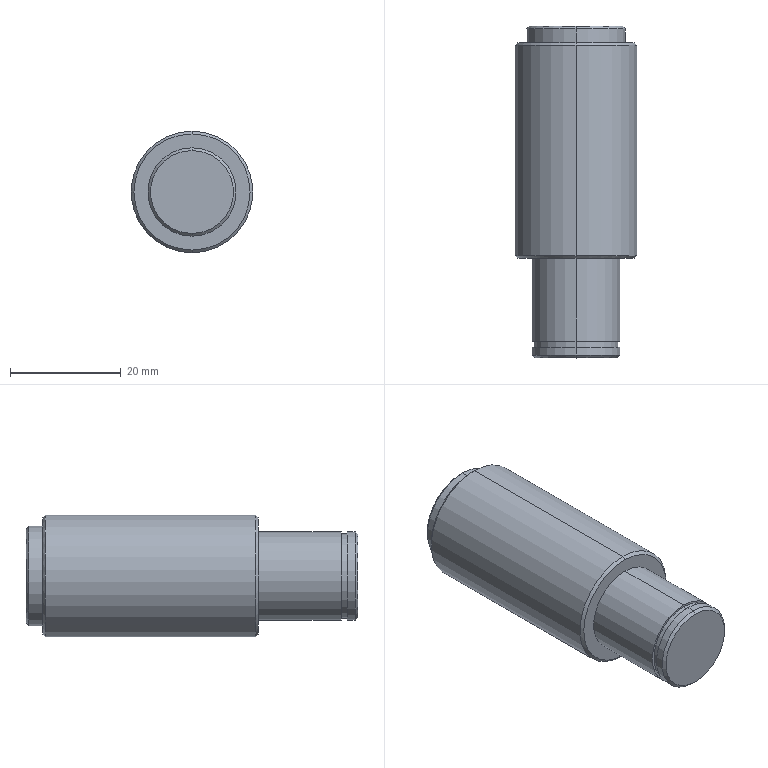Part | STEP file | 02-Support shaft 21 | 1 solid | 24 faces | box 22 x 60 x 22 mm | volume 19156 mm3 | cylinder 10 | cone 8 | plane 6 | commonest cylinder face diameters 16 x4 15.2 x2 18 x2 22 x2
STEP:
#1=CARTESIAN_POINT('',(0.,0.,0.));
#2=DIRECTION('',(0.,0.,1.));
#3=DIRECTION('',(1.,0.,0.));
#4=AXIS2_PLACEMENT_3D('',#1,#2,#3);
#5=CARTESIAN_POINT('',(0.,0.,8.5));
#6=VERTEX_POINT('',#5);
#7=CARTESIAN_POINT('',(0.,0.,-8.5));
#8=VERTEX_POINT('',#7);
#9=CARTESIAN_POINT('',(0.,0.,0.));
#10=DIRECTION('',(0.,1.,0.));
#11=DIRECTION('',(0.,0.,1.));
#12=AXIS2_PLACEMENT_3D('',#9,#10,#11);
#13=CIRCLE('',#12,8.5);
#14=CARTESIAN_POINT('',(0.,0.,0.));
#15=DIRECTION('',(0.,-1.,0.));
#16=DIRECTION('',(0.,0.,-1.));
#17=AXIS2_PLACEMENT_3D('',#14,#15,#16);
#18=CONICAL_SURFACE('',#17,8.5,0.7854);
#19=CARTESIAN_POINT('',(3.142,0.));
#20=DIRECTION('',(-1.,0.));
#21=VECTOR('',#20,1.);
#22=LINE('',#19,#21);
#23=(GEOMETRIC_REPRESENTATION_CONTEXT(2)PARAMETRIC_REPRESENTATION_CONTEXT()REPRESENTATION_CONTEXT('',''));
#24=DEFINITIONAL_REPRESENTATION('',(#22),#23);
#25=PCURVE('',#18,#24);
#26=CARTESIAN_POINT('',(0.,0.,0.));
#27=DIRECTION('',(0.,1.,0.));
#28=DIRECTION('',(0.,0.,1.));
#29=AXIS2_PLACEMENT_3D('',#26,#27,#28);
#30=PLANE('',#29);
#31=CARTESIAN_POINT('',(0.,0.));
#32=DIRECTION('',(1.,0.));
#33=AXIS2_PLACEMENT_2D('',#31,#32);
#34=CIRCLE('',#33,8.5);
#35=(GEOMETRIC_REPRESENTATION_CONTEXT(2)PARAMETRIC_REPRESENTATION_CONTEXT()REPRESENTATION_CONTEXT('',''));
#36=DEFINITIONAL_REPRESENTATION('',(#34),#35);
#37=PCURVE('',#30,#36);
#38=SURFACE_CURVE('',#13,(#25,#37),.PCURVE_S1.);
#39=EDGE_CURVE('',#6,#8,#38,.T.);
#40=ORIENTED_EDGE('',*,*,#39,.F.);
#41=CARTESIAN_POINT('',(0.,-0.5,9.));
#42=VERTEX_POINT('',#41);
#43=CARTESIAN_POINT('',(0.,0.,8.5));
#44=DIRECTION('',(0.,-0.7071,0.7071));
#45=VECTOR('',#44,1.);
#46=LINE('',#43,#45);
#47=CARTESIAN_POINT('',(3.142,0.));
#48=DIRECTION('',(0.,1.));
#49=VECTOR('',#48,1.);
#50=LINE('',#47,#49);
#51=(GEOMETRIC_REPRESENTATION_CONTEXT(2)PARAMETRIC_REPRESENTATION_CONTEXT()REPRESENTATION_CONTEXT('',''));
#52=DEFINITIONAL_REPRESENTATION('',(#50),#51);
#53=PCURVE('',#18,#52);
#54=CARTESIAN_POINT('',(0.,0.,0.));
#55=DIRECTION('',(0.,-1.,0.));
#56=DIRECTION('',(0.,0.,-1.));
#57=AXIS2_PLACEMENT_3D('',#54,#55,#56);
#58=CONICAL_SURFACE('',#57,8.5,0.7854);
#59=CARTESIAN_POINT('',(3.142,0.));
#60=DIRECTION('',(0.,1.));
#61=VECTOR('',#60,1.);
#62=LINE('',#59,#61);
#63=(GEOMETRIC_REPRESENTATION_CONTEXT(2)PARAMETRIC_REPRESENTATION_CONTEXT()REPRESENTATION_CONTEXT('',''));
#64=DEFINITIONAL_REPRESENTATION('',(#62),#63);
#65=PCURVE('',#58,#64);
#66=SURFACE_CURVE('',#46,(#53,#65),.PCURVE_S1.);
#67=EDGE_CURVE('',#6,#42,#66,.T.);
#68=ORIENTED_EDGE('',*,*,#67,.T.);
#69=CARTESIAN_POINT('',(0.,-0.5,-9.));
#70=VERTEX_POINT('',#69);
#71=CARTESIAN_POINT('',(0.,-0.5,0.));
#72=DIRECTION('',(0.,-1.,0.));
#73=DIRECTION('',(0.,0.,1.));
#74=AXIS2_PLACEMENT_3D('',#71,#72,#73);
#75=CIRCLE('',#74,9.);
#76=CARTESIAN_POINT('',(-3.142,0.5));
#77=DIRECTION('',(1.,0.));
#78=VECTOR('',#77,1.);
#79=LINE('',#76,#78);
#80=(GEOMETRIC_REPRESENTATION_CONTEXT(2)PARAMETRIC_REPRESENTATION_CONTEXT()REPRESENTATION_CONTEXT('',''));
#81=DEFINITIONAL_REPRESENTATION('',(#79),#80);
#82=PCURVE('',#18,#81);
#83=CARTESIAN_POINT('',(0.,0.,0.));
#84=DIRECTION('',(0.,1.,0.));
#85=DIRECTION('',(0.,0.,1.));
#86=AXIS2_PLACEMENT_3D('',#83,#84,#85);
#87=CYLINDRICAL_SURFACE('',#86,9.);
#88=CARTESIAN_POINT('',(6.283,-0.5));
#89=DIRECTION('',(-1.,0.));
#90=VECTOR('',#89,1.);
#91=LINE('',#88,#90);
#92=(GEOMETRIC_REPRESENTATION_CONTEXT(2)PARAMETRIC_REPRESENTATION_CONTEXT()REPRESENTATION_CONTEXT('',''));
#93=DEFINITIONAL_REPRESENTATION('',(#91),#92);
#94=PCURVE('',#87,#93);
#95=SURFACE_CURVE('',#75,(#82,#94),.PCURVE_S1.);
#96=EDGE_CURVE('',#70,#42,#95,.T.);
#97=ORIENTED_EDGE('',*,*,#96,.F.);
#98=CARTESIAN_POINT('',(0.,0.,-8.5));
#99=DIRECTION('',(0.,-0.7071,-0.7071));
#100=VECTOR('',#99,1.);
#101=LINE('',#98,#100);
#102=CARTESIAN_POINT('',(0.,0.));
#103=DIRECTION('',(0.,1.));
#104=VECTOR('',#103,1.);
#105=LINE('',#102,#104);
#106=(GEOMETRIC_REPRESENTATION_CONTEXT(2)PARAMETRIC_REPRESENTATION_CONTEXT()REPRESENTATION_CONTEXT('',''));
#107=DEFINITIONAL_REPRESENTATION('',(#105),#106);
#108=PCURVE('',#18,#107);
#109=CARTESIAN_POINT('',(6.283,0.));
#110=DIRECTION('',(0.,1.));
#111=VECTOR('',#110,1.);
#112=LINE('',#109,#111);
#113=(GEOMETRIC_REPRESENTATION_CONTEXT(2)PARAMETRIC_REPRESENTATION_CONTEXT()REPRESENTATION_CONTEXT('',''));
#114=DEFINITIONAL_REPRESENTATION('',(#112),#113);
#115=PCURVE('',#58,#114);
#116=SURFACE_CURVE('',#101,(#108,#115),.PCURVE_S1.);
#117=EDGE_CURVE('',#8,#70,#116,.T.);
#118=ORIENTED_EDGE('',*,*,#117,.F.);
#119=EDGE_LOOP('',(#40,#68,#97,#118));
#120=FACE_BOUND('',#119,.T.);
#121=ADVANCED_FACE('',(#120),#18,.T.);
#122=CARTESIAN_POINT('',(0.,-3.,10.5));
#123=VERTEX_POINT('',#122);
#124=CARTESIAN_POINT('',(0.,-3.,-10.5));
#125=VERTEX_POINT('',#124);
#126=CARTESIAN_POINT('',(0.,-3.,0.));
#127=DIRECTION('',(0.,1.,0.));
#128=DIRECTION('',(0.,0.,1.));
#129=AXIS2_PLACEMENT_3D('',#126,#127,#128);
#130=CIRCLE('',#129,10.5);
#131=CARTESIAN_POINT('',(0.,-3.,0.));
#132=DIRECTION('',(0.,-1.,0.));
#133=DIRECTION('',(0.,0.,-1.));
#134=AXIS2_PLACEMENT_3D('',#131,#132,#133);
#135=CONICAL_SURFACE('',#134,10.5,0.7854);
#136=CARTESIAN_POINT('',(3.142,0.));
#137=DIRECTION('',(-1.,0.));
#138=VECTOR('',#137,1.);
#139=LINE('',#136,#138);
#140=(GEOMETRIC_REPRESENTATION_CONTEXT(2)PARAMETRIC_REPRESENTATION_CONTEXT()REPRESENTATION_CONTEXT('',''));
#141=DEFINITIONAL_REPRESENTATION('',(#139),#140);
#142=PCURVE('',#135,#141);
#143=CARTESIAN_POINT('',(-9.,-3.,0.));
#144=DIRECTION('',(0.,1.,0.));
#145=DIRECTION('',(0.,0.,1.));
#146=AXIS2_PLACEMENT_3D('',#143,#144,#145);
#147=PLANE('',#146);
#148=CARTESIAN_POINT('',(0.,9.));
#149=DIRECTION('',(1.,0.));
#150=AXIS2_PLACEMENT_2D('',#148,#149);
#151=CIRCLE('',#150,10.5);
#152=(GEOMETRIC_REPRESENTATION_CONTEXT(2)PARAMETRIC_REPRESENTATION_CONTEXT()REPRESENTATION_CONTEXT('',''));
#153=DEFINITIONAL_REPRESENTATION('',(#151),#152);
#154=PCURVE('',#147,#153);
#155=SURFACE_CURVE('',#130,(#142,#154),.PCURVE_S1.);
#156=EDGE_CURVE('',#123,#125,#155,.T.);
#157=ORIENTED_EDGE('',*,*,#156,.F.);
#158=CARTESIAN_POINT('',(0.,-3.5,11.));
#159=VERTEX_POINT('',#158);
#160=CARTESIAN_POINT('',(0.,-3.,10.5));
#161=DIRECTION('',(0.,-0.7071,0.7071));
#162=VECTOR('',#161,1.);
#163=LINE('',#160,#162);
#164=CARTESIAN_POINT('',(3.142,0.));
#165=DIRECTION('',(0.,1.));
#166=VECTOR('',#165,1.);
#167=LINE('',#164,#166);
#168=(GEOMETRIC_REPRESENTATION_CONTEXT(2)PARAMETRIC_REPRESENTATION_CONTEXT()REPRESENTATION_CONTEXT('',''));
#169=DEFINITIONAL_REPRESENTATION('',(#167),#168);
#170=PCURVE('',#135,#169);
#171=CARTESIAN_POINT('',(0.,-3.,0.));
#172=DIRECTION('',(0.,-1.,0.));
#173=DIRECTION('',(0.,0.,-1.));
#174=AXIS2_PLACEMENT_3D('',#171,#172,#173);
#175=CONICAL_SURFACE('',#174,10.5,0.7854);
#176=CARTESIAN_POINT('',(3.142,0.));
#177=DIRECTION('',(0.,1.));
#178=VECTOR('',#177,1.);
#179=LINE('',#176,#178);
#180=(GEOMETRIC_REPRESENTATION_CONTEXT(2)PARAMETRIC_REPRESENTATION_CONTEXT()REPRESENTATION_CONTEXT('',''));
#181=DEFINITIONAL_REPRESENTATION('',(#179),#180);
#182=PCURVE('',#175,#181);
#183=SURFACE_CURVE('',#163,(#170,#182),.PCURVE_S1.);
#184=EDGE_CURVE('',#123,#159,#183,.T.);
#185=ORIENTED_EDGE('',*,*,#184,.T.);
#186=CARTESIAN_POINT('',(0.,-3.5,-11.));
#187=VERTEX_POINT('',#186);
#188=CARTESIAN_POINT('',(0.,-3.5,0.));
#189=DIRECTION('',(0.,-1.,0.));
#190=DIRECTION('',(0.,0.,1.));
#191=AXIS2_PLACEMENT_3D('',#188,#189,#190);
#192=CIRCLE('',#191,11.);
#193=CARTESIAN_POINT('',(-3.142,0.5));
#194=DIRECTION('',(1.,0.));
#195=VECTOR('',#194,1.);
#196=LINE('',#193,#195);
#197=(GEOMETRIC_REPRESENTATION_CONTEXT(2)PARAMETRIC_REPRESENTATION_CONTEXT()REPRESENTATION_CONTEXT('',''));
#198=DEFINITIONAL_REPRESENTATION('',(#196),#197);
#199=PCURVE('',#135,#198);
#200=CARTESIAN_POINT('',(0.,0.,0.));
#201=DIRECTION('',(0.,1.,0.));
#202=DIRECTION('',(0.,0.,1.));
#203=AXIS2_PLACEMENT_3D('',#200,#201,#202);
#204=CYLINDRICAL_SURFACE('',#203,11.);
#205=CARTESIAN_POINT('',(6.283,-3.5));
#206=DIRECTION('',(-1.,0.));
#207=VECTOR('',#206,1.);
#208=LINE('',#205,#207);
#209=(GEOMETRIC_REPRESENTATION_CONTEXT(2)PARAMETRIC_REPRESENTATION_CONTEXT()REPRESENTATION_CONTEXT('',''));
#210=DEFINITIONAL_REPRESENTATION('',(#208),#209);
#211=PCURVE('',#204,#210);
#212=SURFACE_CURVE('',#192,(#199,#211),.PCURVE_S1.);
#213=EDGE_CURVE('',#187,#159,#212,.T.);
#214=ORIENTED_EDGE('',*,*,#213,.F.);
#215=CARTESIAN_POINT('',(0.,-3.,-10.5));
#216=DIRECTION('',(0.,-0.7071,-0.7071));
#217=VECTOR('',#216,1.);
#218=LINE('',#215,#217);
#219=CARTESIAN_POINT('',(0.,0.));
#220=DIRECTION('',(0.,1.));
#221=VECTOR('',#220,1.);
#222=LINE('',#219,#221);
#223=(GEOMETRIC_REPRESENTATION_CONTEXT(2)PARAMETRIC_REPRESENTATION_CONTEXT()REPRESENTATION_CONTEXT('',''));
#224=DEFINITIONAL_REPRESENTATION('',(#222),#223);
#225=PCURVE('',#135,#224);
#226=CARTESIAN_POINT('',(6.283,0.));
#227=DIRECTION('',(0.,1.));
#228=VECTOR('',#227,1.);
#229=LINE('',#226,#228);
#230=(GEOMETRIC_REPRESENTATION_CONTEXT(2)PARAMETRIC_REPRESENTATION_CONTEXT()REPRESENTATION_CONTEXT('',''));
#231=DEFINITIONAL_REPRESENTATION('',(#229),#230);
#232=PCURVE('',#175,#231);
#233=SURFACE_CURVE('',#218,(#225,#232),.PCURVE_S1.);
#234=EDGE_CURVE('',#125,#187,#233,.T.);
#235=ORIENTED_EDGE('',*,*,#234,.F.);
#236=EDGE_LOOP('',(#157,#185,#214,#235));
#237=FACE_BOUND('',#236,.T.);
#238=ADVANCED_FACE('',(#237),#135,.T.);
#239=CARTESIAN_POINT('',(0.,-42.,-10.5));
#240=VERTEX_POINT('',#239);
#241=CARTESIAN_POINT('',(0.,-42.,10.5));
#242=VERTEX_POINT('',#241);
#243=CARTESIAN_POINT('',(0.,-42.,0.));
#244=DIRECTION('',(0.,-1.,0.));
#245=DIRECTION('',(0.,0.,-1.));
#246=AXIS2_PLACEMENT_3D('',#243,#244,#245);
#247=CIRCLE('',#246,10.5);
#248=CARTESIAN_POINT('',(0.,-41.5,0.));
#249=DIRECTION('',(0.,1.,0.));
#250=DIRECTION('',(0.,0.,1.));
#251=AXIS2_PLACEMENT_3D('',#248,#249,#250);
#252=CONICAL_SURFACE('',#251,11.,0.7854);
#253=CARTESIAN_POINT('',(3.142,-0.5));
#254=DIRECTION('',(-1.,0.));
#255=VECTOR('',#254,1.);
#256=LINE('',#253,#255);
#257=(GEOMETRIC_REPRESENTATION_CONTEXT(2)PARAMETRIC_REPRESENTATION_CONTEXT()REPRESENTATION_CONTEXT('',''));
#258=DEFINITIONAL_REPRESENTATION('',(#256),#257);
#259=PCURVE('',#252,#258);
#260=CARTESIAN_POINT('',(-11.,-42.,0.));
#261=DIRECTION('',(0.,-1.,0.));
#262=DIRECTION('',(0.,0.,-1.));
#263=AXIS2_PLACEMENT_3D('',#260,#261,#262);
#264=PLANE('',#263);
#265=CARTESIAN_POINT('',(0.,11.));
#266=DIRECTION('',(1.,0.));
#267=AXIS2_PLACEMENT_2D('',#265,#266);
#268=CIRCLE('',#267,10.5);
#269=(GEOMETRIC_REPRESENTATION_CONTEXT(2)PARAMETRIC_REPRESENTATION_CONTEXT()REPRESENTATION_CONTEXT('',''));
#270=DEFINITIONAL_REPRESENTATION('',(#268),#269);
#271=PCURVE('',#264,#270);
#272=SURFACE_CURVE('',#247,(#259,#271),.PCURVE_S1.);
#273=EDGE_CURVE('',#240,#242,#272,.T.);
#274=ORIENTED_EDGE('',*,*,#273,.F.);
#275=CARTESIAN_POINT('',(0.,-41.5,-11.));
#276=VERTEX_POINT('',#275);
#277=CARTESIAN_POINT('',(0.,-41.5,-11.));
#278=DIRECTION('',(0.,0.7071,-0.7071));
#279=VECTOR('',#278,1.);
#280=LINE('',#277,#279);
#281=CARTESIAN_POINT('',(3.142,0.));
#282=DIRECTION('',(0.,1.));
#283=VECTOR('',#282,1.);
#284=LINE('',#281,#283);
#285=(GEOMETRIC_REPRESENTATION_CONTEXT(2)PARAMETRIC_REPRESENTATION_CONTEXT()REPRESENTATION_CONTEXT('',''));
#286=DEFINITIONAL_REPRESENTATION('',(#284),#285);
#287=PCURVE('',#252,#286);
#288=CARTESIAN_POINT('',(0.,-41.5,0.));
#289=DIRECTION('',(0.,1.,0.));
#290=DIRECTION('',(0.,0.,1.));
#291=AXIS2_PLACEMENT_3D('',#288,#289,#290);
#292=CONICAL_SURFACE('',#291,11.,0.7854);
#293=CARTESIAN_POINT('',(3.142,0.));
#294=DIRECTION('',(0.,1.));
#295=VECTOR('',#294,1.);
#296=LINE('',#293,#295);
#297=(GEOMETRIC_REPRESENTATION_CONTEXT(2)PARAMETRIC_REPRESENTATION_CONTEXT()REPRESENTATION_CONTEXT('',''));
#298=DEFINITIONAL_REPRESENTATION('',(#296),#297);
#299=PCURVE('',#292,#298);
#300=SURFACE_CURVE('',#280,(#287,#299),.PCURVE_S1.);
#301=EDGE_CURVE('',#240,#276,#300,.T.);
#302=ORIENTED_EDGE('',*,*,#301,.T.);
#303=CARTESIAN_POINT('',(0.,-41.5,11.));
#304=VERTEX_POINT('',#303);
#305=CARTESIAN_POINT('',(0.,-41.5,0.));
#306=DIRECTION('',(0.,1.,0.));
#307=DIRECTION('',(0.,0.,-1.));
#308=AXIS2_PLACEMENT_3D('',#305,#306,#307);
#309=CIRCLE('',#308,11.);
#310=CARTESIAN_POINT('',(-3.142,0.));
#311=DIRECTION('',(1.,0.));
#312=VECTOR('',#311,1.);
#313=LINE('',#310,#312);
#314=(GEOMETRIC_REPRESENTATION_CONTEXT(2)PARAMETRIC_REPRESENTATION_CONTEXT()REPRESENTATION_CONTEXT('',''));
#315=DEFINITIONAL_REPRESENTATION('',(#313),#314);
#316=PCURVE('',#252,#315);
#317=CARTESIAN_POINT('',(-3.142,-41.5));
#318=DIRECTION('',(1.,0.));
#319=VECTOR('',#318,1.);
#320=LINE('',#317,#319);
#321=(GEOMETRIC_REPRESENTATION_CONTEXT(2)PARAMETRIC_REPRESENTATION_CONTEXT()REPRESENTATION_CONTEXT('',''));
#322=DEFINITIONAL_REPRESENTATION('',(#320),#321);
#323=PCURVE('',#204,#322);
#324=SURFACE_CURVE('',#309,(#316,#323),.PCURVE_S1.);
#325=EDGE_CURVE('',#304,#276,#324,.T.);
#326=ORIENTED_EDGE('',*,*,#325,.F.);
#327=CARTESIAN_POINT('',(0.,-41.5,11.));
#328=DIRECTION('',(0.,0.7071,0.7071));
#329=VECTOR('',#328,1.);
#330=LINE('',#327,#329);
#331=CARTESIAN_POINT('',(0.,0.));
#332=DIRECTION('',(0.,1.));
#333=VECTOR('',#332,1.);
#334=LINE('',#331,#333);
#335=(GEOMETRIC_REPRESENTATION_CONTEXT(2)PARAMETRIC_REPRESENTATION_CONTEXT()REPRESENTATION_CONTEXT('',''));
#336=DEFINITIONAL_REPRESENTATION('',(#334),#335);
#337=PCURVE('',#252,#336);
#338=CARTESIAN_POINT('',(6.283,0.));
#339=DIRECTION('',(0.,1.));
#340=VECTOR('',#339,1.);
#341=LINE('',#338,#340);
#342=(GEOMETRIC_REPRESENTATION_CONTEXT(2)PARAMETRIC_REPRESENTATION_CONTEXT()REPRESENTATION_CONTEXT('',''));
#343=DEFINITIONAL_REPRESENTATION('',(#341),#342);
#344=PCURVE('',#292,#343);
#345=SURFACE_CURVE('',#330,(#337,#344),.PCURVE_S1.);
#346=EDGE_CURVE('',#242,#304,#345,.T.);
#347=ORIENTED_EDGE('',*,*,#346,.F.);
#348=EDGE_LOOP('',(#274,#302,#326,#347));
#349=FACE_BOUND('',#348,.T.);
#350=ADVANCED_FACE('',(#349),#252,.T.);
#351=CARTESIAN_POINT('',(0.,-60.,-7.5));
#352=VERTEX_POINT('',#351);
#353=CARTESIAN_POINT('',(0.,-60.,7.5));
#354=VERTEX_POINT('',#353);
#355=CARTESIAN_POINT('',(0.,-60.,0.));
#356=DIRECTION('',(0.,-1.,0.));
#357=DIRECTION('',(0.,0.,-1.));
#358=AXIS2_PLACEMENT_3D('',#355,#356,#357);
#359=CIRCLE('',#358,7.5);
#360=CARTESIAN_POINT('',(0.,-59.5,0.));
#361=DIRECTION('',(0.,1.,0.));
#362=DIRECTION('',(0.,0.,1.));
#363=AXIS2_PLACEMENT_3D('',#360,#361,#362);
#364=CONICAL_SURFACE('',#363,8.,0.7854);
#365=CARTESIAN_POINT('',(3.142,-0.5));
#366=DIRECTION('',(-1.,0.));
#367=VECTOR('',#366,1.);
#368=LINE('',#365,#367);
#369=(GEOMETRIC_REPRESENTATION_CONTEXT(2)PARAMETRIC_REPRESENTATION_CONTEXT()REPRESENTATION_CONTEXT('',''));
#370=DEFINITIONAL_REPRESENTATION('',(#368),#369);
#371=PCURVE('',#364,#370);
#372=CARTESIAN_POINT('',(-8.,-60.,0.));
#373=DIRECTION('',(0.,-1.,0.));
#374=DIRECTION('',(0.,0.,-1.));
#375=AXIS2_PLACEMENT_3D('',#372,#373,#374);
#376=PLANE('',#375);
#377=CARTESIAN_POINT('',(0.,8.));
#378=DIRECTION('',(1.,0.));
#379=AXIS2_PLACEMENT_2D('',#377,#378);
#380=CIRCLE('',#379,7.5);
#381=(GEOMETRIC_REPRESENTATION_CONTEXT(2)PARAMETRIC_REPRESENTATION_CONTEXT()REPRESENTATION_CONTEXT('',''));
#382=DEFINITIONAL_REPRESENTATION('',(#380),#381);
#383=PCURVE('',#376,#382);
#384=SURFACE_CURVE('',#359,(#371,#383),.PCURVE_S1.);
#385=EDGE_CURVE('',#352,#354,#384,.T.);
#386=ORIENTED_EDGE('',*,*,#385,.F.);
#387=CARTESIAN_POINT('',(0.,-59.5,-8.));
#388=VERTEX_POINT('',#387);
#389=CARTESIAN_POINT('',(0.,-59.5,-8.));
#390=DIRECTION('',(0.,0.7071,-0.7071));
#391=VECTOR('',#390,1.);
#392=LINE('',#389,#391);
#393=CARTESIAN_POINT('',(3.142,0.));
#394=DIRECTION('',(0.,1.));
#395=VECTOR('',#394,1.);
#396=LINE('',#393,#395);
#397=(GEOMETRIC_REPRESENTATION_CONTEXT(2)PARAMETRIC_REPRESENTATION_CONTEXT()REPRESENTATION_CONTEXT('',''));
#398=DEFINITIONAL_REPRESENTATION('',(#396),#397);
#399=PCURVE('',#364,#398);
#400=CARTESIAN_POINT('',(0.,-59.5,0.));
#401=DIRECTION('',(0.,1.,0.));
#402=DIRECTION('',(0.,0.,1.));
#403=AXIS2_PLACEMENT_3D('',#400,#401,#402);
#404=CONICAL_SURFACE('',#403,8.,0.7854);
#405=CARTESIAN_POINT('',(3.142,0.));
#406=DIRECTION('',(0.,1.));
#407=VECTOR('',#406,1.);
#408=LINE('',#405,#407);
#409=(GEOMETRIC_REPRESENTATION_CONTEXT(2)PARAMETRIC_REPRESENTATION_CONTEXT()REPRESENTATION_CONTEXT('',''));
#410=DEFINITIONAL_REPRESENTATION('',(#408),#409);
#411=PCURVE('',#404,#410);
#412=SURFACE_CURVE('',#392,(#399,#411),.PCURVE_S1.);
#413=EDGE_CURVE('',#352,#388,#412,.T.);
#414=ORIENTED_EDGE('',*,*,#413,.T.);
#415=CARTESIAN_POINT('',(0.,-59.5,8.));
#416=VERTEX_POINT('',#415);
#417=CARTESIAN_POINT('',(0.,-59.5,0.));
#418=DIRECTION('',(0.,1.,0.));
#419=DIRECTION('',(0.,0.,-1.));
#420=AXIS2_PLACEMENT_3D('',#417,#418,#419);
#421=CIRCLE('',#420,8.);
#422=CARTESIAN_POINT('',(-3.142,0.));
#423=DIRECTION('',(1.,0.));
#424=VECTOR('',#423,1.);
#425=LINE('',#422,#424);
#426=(GEOMETRIC_REPRESENTATION_CONTEXT(2)PARAMETRIC_REPRESENTATION_CONTEXT()REPRESENTATION_CONTEXT('',''));
#427=DEFINITIONAL_REPRESENTATION('',(#425),#426);
#428=PCURVE('',#364,#427);
#429=CARTESIAN_POINT('',(0.,0.,0.));
#430=DIRECTION('',(0.,1.,0.));
#431=DIRECTION('',(0.,0.,1.));
#432=AXIS2_PLACEMENT_3D('',#429,#430,#431);
#433=CYLINDRICAL_SURFACE('',#432,8.);
#434=CARTESIAN_POINT('',(-3.142,-59.5));
#435=DIRECTION('',(1.,0.));
#436=VECTOR('',#435,1.);
#437=LINE('',#434,#436);
#438=(GEOMETRIC_REPRESENTATION_CONTEXT(2)PARAMETRIC_REPRESENTATION_CONTEXT()REPRESENTATION_CONTEXT('',''));
#439=DEFINITIONAL_REPRESENTATION('',(#437),#438);
#440=PCURVE('',#433,#439);
#441=SURFACE_CURVE('',#421,(#428,#440),.PCURVE_S1.);
#442=EDGE_CURVE('',#416,#388,#441,.T.);
#443=ORIENTED_EDGE('',*,*,#442,.F.);
#444=CARTESIAN_POINT('',(0.,-59.5,8.));
#445=DIRECTION('',(0.,0.7071,0.7071));
#446=VECTOR('',#445,1.);
#447=LINE('',#444,#446);
#448=CARTESIAN_POINT('',(0.,0.));
#449=DIRECTION('',(0.,1.));
#450=VECTOR('',#449,1.);
#451=LINE('',#448,#450);
#452=(GEOMETRIC_REPRESENTATION_CONTEXT(2)PARAMETRIC_REPRESENTATION_CONTEXT()REPRESENTATION_CONTEXT('',''));
#453=DEFINITIONAL_REPRESENTATION('',(#451),#452);
#454=PCURVE('',#364,#453);
#455=CARTESIAN_POINT('',(6.283,0.));
#456=DIRECTION('',(0.,1.));
#457=VECTOR('',#456,1.);
#458=LINE('',#455,#457);
#459=(GEOMETRIC_REPRESENTATION_CONTEXT(2)PARAMETRIC_REPRESENTATION_CONTEXT()REPRESENTATION_CONTEXT('',''));
#460=DEFINITIONAL_REPRESENTATION('',(#458),#459);
#461=PCURVE('',#404,#460);
#462=SURFACE_CURVE('',#447,(#454,#461),.PCURVE_S1.);
#463=EDGE_CURVE('',#354,#416,#462,.T.);
#464=ORIENTED_EDGE('',*,*,#463,.F.);
#465=EDGE_LOOP('',(#386,#414,#443,#464));
#466=FACE_BOUND('',#465,.T.);
#467=ADVANCED_FACE('',(#466),#364,.T.);
#468=ORIENTED_EDGE('',*,*,#442,.T.);
#469=CARTESIAN_POINT('',(0.,-58.1,-8.));
#470=VERTEX_POINT('',#469);
#471=CARTESIAN_POINT('',(0.,0.,-8.));
#472=DIRECTION('',(0.,1.,0.));
#473=VECTOR('',#472,1.);
#474=LINE('',#471,#473);
#475=CARTESIAN_POINT('',(3.142,0.));
#476=DIRECTION('',(0.,1.));
#477=VECTOR('',#476,1.);
#478=LINE('',#475,#477);
#479=(GEOMETRIC_REPRESENTATION_CONTEXT(2)PARAMETRIC_REPRESENTATION_CONTEXT()REPRESENTATION_CONTEXT('',''));
#480=DEFINITIONAL_REPRESENTATION('',(#478),#479);
#481=PCURVE('',#433,#480);
#482=CARTESIAN_POINT('',(0.,0.,0.));
#483=DIRECTION('',(0.,1.,0.));
#484=DIRECTION('',(0.,0.,1.));
#485=AXIS2_PLACEMENT_3D('',#482,#483,#484);
#486=CYLINDRICAL_SURFACE('',#485,8.);
#487=CARTESIAN_POINT('',(3.142,0.));
#488=DIRECTION('',(0.,1.));
#489=VECTOR('',#488,1.);
#490=LINE('',#487,#489);
#491=(GEOMETRIC_REPRESENTATION_CONTEXT(2)PARAMETRIC_REPRESENTATION_CONTEXT()REPRESENTATION_CONTEXT('',''));
#492=DEFINITIONAL_REPRESENTATION('',(#490),#491);
#493=PCURVE('',#486,#492);
#494=SURFACE_CURVE('',#474,(#481,#493),.PCURVE_S1.);
#495=EDGE_CURVE('',#388,#470,#494,.T.);
#496=ORIENTED_EDGE('',*,*,#495,.T.);
#497=CARTESIAN_POINT('',(0.,-58.1,8.));
#498=VERTEX_POINT('',#497);
#499=CARTESIAN_POINT('',(0.,-58.1,0.));
#500=DIRECTION('',(0.,1.,0.));
#501=DIRECTION('',(0.,0.,1.));
#502=AXIS2_PLACEMENT_3D('',#499,#500,#501);
#503=CIRCLE('',#502,8.);
#504=CARTESIAN_POINT('',(0.,-58.1));
#505=DIRECTION('',(1.,0.));
#506=VECTOR('',#505,1.);
#507=LINE('',#504,#506);
#508=(GEOMETRIC_REPRESENTATION_CONTEXT(2)PARAMETRIC_REPRESENTATION_CONTEXT()REPRESENTATION_CONTEXT('',''));
#509=DEFINITIONAL_REPRESENTATION('',(#507),#508);
#510=PCURVE('',#433,#509);
#511=CARTESIAN_POINT('',(-7.6,-58.1,0.));
#512=DIRECTION('',(0.,1.,0.));
#513=DIRECTION('',(0.,0.,1.));
#514=AXIS2_PLACEMENT_3D('',#511,#512,#513);
#515=PLANE('',#514);
#516=CARTESIAN_POINT('',(0.,7.6));
#517=DIRECTION('',(1.,0.));
#518=AXIS2_PLACEMENT_2D('',#516,#517);
#519=CIRCLE('',#518,8.);
#520=(GEOMETRIC_REPRESENTATION_CONTEXT(2)PARAMETRIC_REPRESENTATION_CONTEXT()REPRESENTATION_CONTEXT('',''));
#521=DEFINITIONAL_REPRESENTATION('',(#519),#520);
#522=PCURVE('',#515,#521);
#523=SURFACE_CURVE('',#503,(#510,#522),.PCURVE_S1.);
#524=EDGE_CURVE('',#498,#470,#523,.T.);
#525=ORIENTED_EDGE('',*,*,#524,.F.);
#526=CARTESIAN_POINT('',(0.,0.,8.));
#527=DIRECTION('',(0.,1.,0.));
#528=VECTOR('',#527,1.);
#529=LINE('',#526,#528);
#530=CARTESIAN_POINT('',(0.,0.));
#531=DIRECTION('',(0.,1.));
#532=VECTOR('',#531,1.);
#533=LINE('',#530,#532);
#534=(GEOMETRIC_REPRESENTATION_CONTEXT(2)PARAMETRIC_REPRESENTATION_CONTEXT()REPRESENTATION_CONTEXT('',''));
#535=DEFINITIONAL_REPRESENTATION('',(#533),#534);
#536=PCURVE('',#433,#535);
#537=CARTESIAN_POINT('',(6.283,0.));
#538=DIRECTION('',(0.,1.));
#539=VECTOR('',#538,1.);
#540=LINE('',#537,#539);
#541=(GEOMETRIC_REPRESENTATION_CONTEXT(2)PARAMETRIC_REPRESENTATION_CONTEXT()REPRESENTATION_CONTEXT('',''));
#542=DEFINITIONAL_REPRESENTATION('',(#540),#541);
#543=PCURVE('',#486,#542);
#544=SURFACE_CURVE('',#529,(#536,#543),.PCURVE_S1.);
#545=EDGE_CURVE('',#416,#498,#544,.T.);
#546=ORIENTED_EDGE('',*,*,#545,.F.);
#547=EDGE_LOOP('',(#468,#496,#525,#546));
#548=FACE_BOUND('',#547,.T.);
#549=ADVANCED_FACE('',(#548),#433,.T.);
#550=CARTESIAN_POINT('',(0.,-58.1,7.6));
#551=VERTEX_POINT('',#550);
#552=CARTESIAN_POINT('',(0.,-58.1,-7.6));
#553=VERTEX_POINT('',#552);
#554=CARTESIAN_POINT('',(0.,-58.1,0.));
#555=DIRECTION('',(0.,1.,0.));
#556=DIRECTION('',(0.,0.,1.));
#557=AXIS2_PLACEMENT_3D('',#554,#555,#556);
#558=CIRCLE('',#557,7.6);
#559=CARTESIAN_POINT('',(0.,0.,0.));
#560=DIRECTION('',(0.,1.,0.));
#561=DIRECTION('',(0.,0.,1.));
#562=AXIS2_PLACEMENT_3D('',#559,#560,#561);
#563=CYLINDRICAL_SURFACE('',#562,7.6);
#564=CARTESIAN_POINT('',(0.,-58.1));
#565=DIRECTION('',(1.,0.));
#566=VECTOR('',#565,1.);
#567=LINE('',#564,#566);
#568=(GEOMETRIC_REPRESENTATION_CONTEXT(2)PARAMETRIC_REPRESENTATION_CONTEXT()REPRESENTATION_CONTEXT('',''));
#569=DEFINITIONAL_REPRESENTATION('',(#567),#568);
#570=PCURVE('',#563,#569);
#571=CARTESIAN_POINT('',(0.,7.6));
#572=DIRECTION('',(1.,0.));
#573=AXIS2_PLACEMENT_2D('',#571,#572);
#574=CIRCLE('',#573,7.6);
#575=(GEOMETRIC_REPRESENTATION_CONTEXT(2)PARAMETRIC_REPRESENTATION_CONTEXT()REPRESENTATION_CONTEXT('',''));
#576=DEFINITIONAL_REPRESENTATION('',(#574),#575);
#577=PCURVE('',#515,#576);
#578=SURFACE_CURVE('',#558,(#570,#577),.PCURVE_S1.);
#579=EDGE_CURVE('',#551,#553,#578,.T.);
#580=ORIENTED_EDGE('',*,*,#579,.T.);
#581=CARTESIAN_POINT('',(0.,-57.,-7.6));
#582=VERTEX_POINT('',#581);
#583=CARTESIAN_POINT('',(0.,0.,-7.6));
#584=DIRECTION('',(0.,1.,0.));
#585=VECTOR('',#584,1.);
#586=LINE('',#583,#585);
#587=CARTESIAN_POINT('',(3.142,0.));
#588=DIRECTION('',(0.,1.));
#589=VECTOR('',#588,1.);
#590=LINE('',#587,#589);
#591=(GEOMETRIC_REPRESENTATION_CONTEXT(2)PARAMETRIC_REPRESENTATION_CONTEXT()REPRESENTATION_CONTEXT('',''));
#592=DEFINITIONAL_REPRESENTATION('',(#590),#591);
#593=PCURVE('',#563,#592);
#594=CARTESIAN_POINT('',(0.,0.,0.));
#595=DIRECTION('',(0.,1.,0.));
#596=DIRECTION('',(0.,0.,1.));
#597=AXIS2_PLACEMENT_3D('',#594,#595,#596);
#598=CYLINDRICAL_SURFACE('',#597,7.6);
#599=CARTESIAN_POINT('',(3.142,0.));
#600=DIRECTION('',(0.,1.));
#601=VECTOR('',#600,1.);
#602=LINE('',#599,#601);
#603=(GEOMETRIC_REPRESENTATION_CONTEXT(2)PARAMETRIC_REPRESENTATION_CONTEXT()REPRESENTATION_CONTEXT('',''));
#604=DEFINITIONAL_REPRESENTATION('',(#602),#603);
#605=PCURVE('',#598,#604);
#606=SURFACE_CURVE('',#586,(#593,#605),.PCURVE_S1.);
#607=EDGE_CURVE('',#553,#582,#606,.T.);
#608=ORIENTED_EDGE('',*,*,#607,.T.);
#609=CARTESIAN_POINT('',(0.,-57.,7.6));
#610=VERTEX_POINT('',#609);
#611=CARTESIAN_POINT('',(0.,-57.,0.));
#612=DIRECTION('',(0.,1.,0.));
#613=DIRECTION('',(0.,0.,1.));
#614=AXIS2_PLACEMENT_3D('',#611,#612,#613);
#615=CIRCLE('',#614,7.6);
#616=CARTESIAN_POINT('',(0.,-57.));
#617=DIRECTION('',(1.,0.));
#618=VECTOR('',#617,1.);
#619=LINE('',#616,#618);
#620=(GEOMETRIC_REPRESENTATION_CONTEXT(2)PARAMETRIC_REPRESENTATION_CONTEXT()REPRESENTATION_CONTEXT('',''));
#621=DEFINITIONAL_REPRESENTATION('',(#619),#620);
#622=PCURVE('',#563,#621);
#623=CARTESIAN_POINT('',(-8.,-57.,0.));
#624=DIRECTION('',(0.,-1.,0.));
#625=DIRECTION('',(0.,0.,-1.));
#626=AXIS2_PLACEMENT_3D('',#623,#624,#625);
#627=PLANE('',#626);
#628=CARTESIAN_POINT('',(-7.6,8.));
#629=CARTESIAN_POINT('',(-7.6,21.164));
#630=CARTESIAN_POINT('',(3.8,14.582));
#631=CARTESIAN_POINT('',(15.2,8.));
#632=CARTESIAN_POINT('',(3.8,1.418));
#633=CARTESIAN_POINT('',(-7.6,-5.164));
#634=CARTESIAN_POINT('',(-7.6,8.));
#635=(BOUNDED_CURVE()B_SPLINE_CURVE(2,(#628,#629,#630,#631,#632,#633,#634),.UNSPECIFIED.,.T.,.F.)B_SPLINE_CURVE_WITH_KNOTS((1,2,2,2,2,1),(-2.094,0.,2.094,4.189,6.283,8.378),.UNSPECIFIED.)CURVE()GEOMETRIC_REPRESENTATION_ITEM()RATIONAL_B_SPLINE_CURVE((1.,0.5,1.,0.5,1.,0.5,1.))REPRESENTATION_ITEM(''));
#636=(GEOMETRIC_REPRESENTATION_CONTEXT(2)PARAMETRIC_REPRESENTATION_CONTEXT()REPRESENTATION_CONTEXT('',''));
#637=DEFINITIONAL_REPRESENTATION('',(#635),#636);
#638=PCURVE('',#627,#637);
#639=SURFACE_CURVE('',#615,(#622,#638),.PCURVE_S1.);
#640=EDGE_CURVE('',#610,#582,#639,.T.);
#641=ORIENTED_EDGE('',*,*,#640,.F.);
#642=CARTESIAN_POINT('',(0.,0.,7.6));
#643=DIRECTION('',(0.,1.,0.));
#644=VECTOR('',#643,1.);
#645=LINE('',#642,#644);
#646=CARTESIAN_POINT('',(0.,0.));
#647=DIRECTION('',(0.,1.));
#648=VECTOR('',#647,1.);
#649=LINE('',#646,#648);
#650=(GEOMETRIC_REPRESENTATION_CONTEXT(2)PARAMETRIC_REPRESENTATION_CONTEXT()REPRESENTATION_CONTEXT('',''));
#651=DEFINITIONAL_REPRESENTATION('',(#649),#650);
#652=PCURVE('',#563,#651);
#653=CARTESIAN_POINT('',(6.283,0.));
#654=DIRECTION('',(0.,1.));
#655=VECTOR('',#654,1.);
#656=LINE('',#653,#655);
#657=(GEOMETRIC_REPRESENTATION_CONTEXT(2)PARAMETRIC_REPRESENTATION_CONTEXT()REPRESENTATION_CONTEXT('',''));
#658=DEFINITIONAL_REPRESENTATION('',(#656),#657);
#659=PCURVE('',#598,#658);
#660=SURFACE_CURVE('',#645,(#652,#659),.PCURVE_S1.);
#661=EDGE_CURVE('',#551,#610,#660,.T.);
#662=ORIENTED_EDGE('',*,*,#661,.F.);
#663=EDGE_LOOP('',(#580,#608,#641,#662));
#664=FACE_BOUND('',#663,.T.);
#665=ADVANCED_FACE('',(#664),#563,.T.);
#666=CARTESIAN_POINT('',(0.,-57.,8.));
#667=VERTEX_POINT('',#666);
#668=CARTESIAN_POINT('',(0.,-57.,-8.));
#669=VERTEX_POINT('',#668);
#670=CARTESIAN_POINT('',(0.,-57.,0.));
#671=DIRECTION('',(0.,1.,0.));
#672=DIRECTION('',(0.,0.,1.));
#673=AXIS2_PLACEMENT_3D('',#670,#671,#672);
#674=CIRCLE('',#673,8.);
#675=CARTESIAN_POINT('',(0.,0.,0.));
#676=DIRECTION('',(0.,1.,0.));
#677=DIRECTION('',(0.,0.,1.));
#678=AXIS2_PLACEMENT_3D('',#675,#676,#677);
#679=CYLINDRICAL_SURFACE('',#678,8.);
#680=CARTESIAN_POINT('',(0.,-57.));
#681=DIRECTION('',(1.,0.));
#682=VECTOR('',#681,1.);
#683=LINE('',#680,#682);
#684=(GEOMETRIC_REPRESENTATION_CONTEXT(2)PARAMETRIC_REPRESENTATION_CONTEXT()REPRESENTATION_CONTEXT('',''));
#685=DEFINITIONAL_REPRESENTATION('',(#683),#684);
#686=PCURVE('',#679,#685);
#687=CARTESIAN_POINT('',(-8.,8.));
#688=CARTESIAN_POINT('',(-8.,21.856));
#689=CARTESIAN_POINT('',(4.,14.928));
#690=CARTESIAN_POINT('',(16.,8.));
#691=CARTESIAN_POINT('',(4.,1.072));
#692=CARTESIAN_POINT('',(-8.,-5.856));
#693=CARTESIAN_POINT('',(-8.,8.));
#694=(BOUNDED_CURVE()B_SPLINE_CURVE(2,(#687,#688,#689,#690,#691,#692,#693),.UNSPECIFIED.,.T.,.F.)B_SPLINE_CURVE_WITH_KNOTS((1,2,2,2,2,1),(-2.094,0.,2.094,4.189,6.283,8.378),.UNSPECIFIED.)CURVE()GEOMETRIC_REPRESENTATION_ITEM()RATIONAL_B_SPLINE_CURVE((1.,0.5,1.,0.5,1.,0.5,1.))REPRESENTATION_ITEM(''));
#695=(GEOMETRIC_REPRESENTATION_CONTEXT(2)PARAMETRIC_REPRESENTATION_CONTEXT()REPRESENTATION_CONTEXT('',''));
#696=DEFINITIONAL_REPRESENTATION('',(#694),#695);
#697=PCURVE('',#627,#696);
#698=SURFACE_CURVE('',#674,(#686,#697),.PCURVE_S1.);
#699=EDGE_CURVE('',#667,#669,#698,.T.);
#700=ORIENTED_EDGE('',*,*,#699,.T.);
#701=CARTESIAN_POINT('',(0.,-42.,-8.));
#702=VERTEX_POINT('',#701);
#703=CARTESIAN_POINT('',(0.,0.,-8.));
#704=DIRECTION('',(0.,1.,0.));
#705=VECTOR('',#704,1.);
#706=LINE('',#703,#705);
#707=CARTESIAN_POINT('',(3.142,0.));
#708=DIRECTION('',(0.,1.));
#709=VECTOR('',#708,1.);
#710=LINE('',#707,#709);
#711=(GEOMETRIC_REPRESENTATION_CONTEXT(2)PARAMETRIC_REPRESENTATION_CONTEXT()REPRESENTATION_CONTEXT('',''));
#712=DEFINITIONAL_REPRESENTATION('',(#710),#711);
#713=PCURVE('',#679,#712);
#714=CARTESIAN_POINT('',(0.,0.,0.));
#715=DIRECTION('',(0.,1.,0.));
#716=DIRECTION('',(0.,0.,1.));
#717=AXIS2_PLACEMENT_3D('',#714,#715,#716);
#718=CYLINDRICAL_SURFACE('',#717,8.);
#719=CARTESIAN_POINT('',(3.142,0.));
#720=DIRECTION('',(0.,1.));
#721=VECTOR('',#720,1.);
#722=LINE('',#719,#721);
#723=(GEOMETRIC_REPRESENTATION_CONTEXT(2)PARAMETRIC_REPRESENTATION_CONTEXT()REPRESENTATION_CONTEXT('',''));
#724=DEFINITIONAL_REPRESENTATION('',(#722),#723);
#725=PCURVE('',#718,#724);
#726=SURFACE_CURVE('',#706,(#713,#725),.PCURVE_S1.);
#727=EDGE_CURVE('',#669,#702,#726,.T.);
#728=ORIENTED_EDGE('',*,*,#727,.T.);
#729=CARTESIAN_POINT('',(0.,-42.,8.));
#730=VERTEX_POINT('',#729);
#731=CARTESIAN_POINT('',(0.,-42.,0.));
#732=DIRECTION('',(0.,1.,0.));
#733=DIRECTION('',(0.,0.,1.));
#734=AXIS2_PLACEMENT_3D('',#731,#732,#733);
#735=CIRCLE('',#734,8.);
#736=CARTESIAN_POINT('',(0.,-42.));
#737=DIRECTION('',(1.,0.));
#738=VECTOR('',#737,1.);
#739=LINE('',#736,#738);
#740=(GEOMETRIC_REPRESENTATION_CONTEXT(2)PARAMETRIC_REPRESENTATION_CONTEXT()REPRESENTATION_CONTEXT('',''));
#741=DEFINITIONAL_REPRESENTATION('',(#739),#740);
#742=PCURVE('',#679,#741);
#743=CARTESIAN_POINT('',(-8.,11.));
#744=CARTESIAN_POINT('',(-8.,24.856));
#745=CARTESIAN_POINT('',(4.,17.928));
#746=CARTESIAN_POINT('',(16.,11.));
#747=CARTESIAN_POINT('',(4.,4.072));
#748=CARTESIAN_POINT('',(-8.,-2.856));
#749=CARTESIAN_POINT('',(-8.,11.));
#750=(BOUNDED_CURVE()B_SPLINE_CURVE(2,(#743,#744,#745,#746,#747,#748,#749),.UNSPECIFIED.,.T.,.F.)B_SPLINE_CURVE_WITH_KNOTS((1,2,2,2,2,1),(-2.094,0.,2.094,4.189,6.283,8.378),.UNSPECIFIED.)CURVE()GEOMETRIC_REPRESENTATION_ITEM()RATIONAL_B_SPLINE_CURVE((1.,0.5,1.,0.5,1.,0.5,1.))REPRESENTATION_ITEM(''));
#751=(GEOMETRIC_REPRESENTATION_CONTEXT(2)PARAMETRIC_REPRESENTATION_CONTEXT()REPRESENTATION_CONTEXT('',''));
#752=DEFINITIONAL_REPRESENTATION('',(#750),#751);
#753=PCURVE('',#264,#752);
#754=SURFACE_CURVE('',#735,(#742,#753),.PCURVE_S1.);
#755=EDGE_CURVE('',#730,#702,#754,.T.);
#756=ORIENTED_EDGE('',*,*,#755,.F.);
#757=CARTESIAN_POINT('',(0.,0.,8.));
#758=DIRECTION('',(0.,1.,0.));
#759=VECTOR('',#758,1.);
#760=LINE('',#757,#759);
#761=CARTESIAN_POINT('',(0.,0.));
#762=DIRECTION('',(0.,1.));
#763=VECTOR('',#762,1.);
#764=LINE('',#761,#763);
#765=(GEOMETRIC_REPRESENTATION_CONTEXT(2)PARAMETRIC_REPRESENTATION_CONTEXT()REPRESENTATION_CONTEXT('',''));
#766=DEFINITIONAL_REPRESENTATION('',(#764),#765);
#767=PCURVE('',#679,#766);
#768=CARTESIAN_POINT('',(6.283,0.));
#769=DIRECTION('',(0.,1.));
#770=VECTOR('',#769,1.);
#771=LINE('',#768,#770);
#772=(GEOMETRIC_REPRESENTATION_CONTEXT(2)PARAMETRIC_REPRESENTATION_CONTEXT()REPRESENTATION_CONTEXT('',''));
#773=DEFINITIONAL_REPRESENTATION('',(#771),#772);
#774=PCURVE('',#718,#773);
#775=SURFACE_CURVE('',#760,(#767,#774),.PCURVE_S1.);
#776=EDGE_CURVE('',#667,#730,#775,.T.);
#777=ORIENTED_EDGE('',*,*,#776,.F.);
#778=EDGE_LOOP('',(#700,#728,#756,#777));
#779=FACE_BOUND('',#778,.T.);
#780=ADVANCED_FACE('',(#779),#679,.T.);
#781=ORIENTED_EDGE('',*,*,#325,.T.);
#782=CARTESIAN_POINT('',(0.,0.,-11.));
#783=DIRECTION('',(0.,1.,0.));
#784=VECTOR('',#783,1.);
#785=LINE('',#782,#784);
#786=CARTESIAN_POINT('',(3.142,0.));
#787=DIRECTION('',(0.,1.));
#788=VECTOR('',#787,1.);
#789=LINE('',#786,#788);
#790=(GEOMETRIC_REPRESENTATION_CONTEXT(2)PARAMETRIC_REPRESENTATION_CONTEXT()REPRESENTATION_CONTEXT('',''));
#791=DEFINITIONAL_REPRESENTATION('',(#789),#790);
#792=PCURVE('',#204,#791);
#793=CARTESIAN_POINT('',(0.,0.,0.));
#794=DIRECTION('',(0.,1.,0.));
#795=DIRECTION('',(0.,0.,1.));
#796=AXIS2_PLACEMENT_3D('',#793,#794,#795);
#797=CYLINDRICAL_SURFACE('',#796,11.);
#798=CARTESIAN_POINT('',(3.142,0.));
#799=DIRECTION('',(0.,1.));
#800=VECTOR('',#799,1.);
#801=LINE('',#798,#800);
#802=(GEOMETRIC_REPRESENTATION_CONTEXT(2)PARAMETRIC_REPRESENTATION_CONTEXT()REPRESENTATION_CONTEXT('',''));
#803=DEFINITIONAL_REPRESENTATION('',(#801),#802);
#804=PCURVE('',#797,#803);
#805=SURFACE_CURVE('',#785,(#792,#804),.PCURVE_S1.);
#806=EDGE_CURVE('',#276,#187,#805,.T.);
#807=ORIENTED_EDGE('',*,*,#806,.T.);
#808=ORIENTED_EDGE('',*,*,#213,.T.);
#809=CARTESIAN_POINT('',(0.,0.,11.));
#810=DIRECTION('',(0.,1.,0.));
#811=VECTOR('',#810,1.);
#812=LINE('',#809,#811);
#813=CARTESIAN_POINT('',(0.,0.));
#814=DIRECTION('',(0.,1.));
#815=VECTOR('',#814,1.);
#816=LINE('',#813,#815);
#817=(GEOMETRIC_REPRESENTATION_CONTEXT(2)PARAMETRIC_REPRESENTATION_CONTEXT()REPRESENTATION_CONTEXT('',''));
#818=DEFINITIONAL_REPRESENTATION('',(#816),#817);
#819=PCURVE('',#204,#818);
#820=CARTESIAN_POINT('',(6.283,0.));
#821=DIRECTION('',(0.,1.));
#822=VECTOR('',#821,1.);
#823=LINE('',#820,#822);
#824=(GEOMETRIC_REPRESENTATION_CONTEXT(2)PARAMETRIC_REPRESENTATION_CONTEXT()REPRESENTATION_CONTEXT('',''));
#825=DEFINITIONAL_REPRESENTATION('',(#823),#824);
#826=PCURVE('',#797,#825);
#827=SURFACE_CURVE('',#812,(#819,#826),.PCURVE_S1.);
#828=EDGE_CURVE('',#304,#159,#827,.T.);
#829=ORIENTED_EDGE('',*,*,#828,.F.);
#830=EDGE_LOOP('',(#781,#807,#808,#829));
#831=FACE_BOUND('',#830,.T.);
#832=ADVANCED_FACE('',(#831),#204,.T.);
#833=CARTESIAN_POINT('',(0.,-3.,9.));
#834=VERTEX_POINT('',#833);
#835=CARTESIAN_POINT('',(0.,-3.,-9.));
#836=VERTEX_POINT('',#835);
#837=CARTESIAN_POINT('',(0.,-3.,0.));
#838=DIRECTION('',(0.,1.,0.));
#839=DIRECTION('',(0.,0.,1.));
#840=AXIS2_PLACEMENT_3D('',#837,#838,#839);
#841=CIRCLE('',#840,9.);
#842=CARTESIAN_POINT('',(0.,-3.));
#843=DIRECTION('',(1.,0.));
#844=VECTOR('',#843,1.);
#845=LINE('',#842,#844);
#846=(GEOMETRIC_REPRESENTATION_CONTEXT(2)PARAMETRIC_REPRESENTATION_CONTEXT()REPRESENTATION_CONTEXT('',''));
#847=DEFINITIONAL_REPRESENTATION('',(#845),#846);
#848=PCURVE('',#87,#847);
#849=CARTESIAN_POINT('',(0.,9.));
#850=DIRECTION('',(1.,0.));
#851=AXIS2_PLACEMENT_2D('',#849,#850);
#852=CIRCLE('',#851,9.);
#853=(GEOMETRIC_REPRESENTATION_CONTEXT(2)PARAMETRIC_REPRESENTATION_CONTEXT()REPRESENTATION_CONTEXT('',''));
#854=DEFINITIONAL_REPRESENTATION('',(#852),#853);
#855=PCURVE('',#147,#854);
#856=SURFACE_CURVE('',#841,(#848,#855),.PCURVE_S1.);
#857=EDGE_CURVE('',#834,#836,#856,.T.);
#858=ORIENTED_EDGE('',*,*,#857,.T.);
#859=CARTESIAN_POINT('',(0.,0.,-9.));
#860=DIRECTION('',(0.,1.,0.));
#861=VECTOR('',#860,1.);
#862=LINE('',#859,#861);
#863=CARTESIAN_POINT('',(3.142,0.));
#864=DIRECTION('',(0.,1.));
#865=VECTOR('',#864,1.);
#866=LINE('',#863,#865);
#867=(GEOMETRIC_REPRESENTATION_CONTEXT(2)PARAMETRIC_REPRESENTATION_CONTEXT()REPRESENTATION_CONTEXT('',''));
#868=DEFINITIONAL_REPRESENTATION('',(#866),#867);
#869=PCURVE('',#87,#868);
#870=CARTESIAN_POINT('',(0.,0.,0.));
#871=DIRECTION('',(0.,1.,0.));
#872=DIRECTION('',(0.,0.,1.));
#873=AXIS2_PLACEMENT_3D('',#870,#871,#872);
#874=CYLINDRICAL_SURFACE('',#873,9.);
#875=CARTESIAN_POINT('',(3.142,0.));
#876=DIRECTION('',(0.,1.));
#877=VECTOR('',#876,1.);
#878=LINE('',#875,#877);
#879=(GEOMETRIC_REPRESENTATION_CONTEXT(2)PARAMETRIC_REPRESENTATION_CONTEXT()REPRESENTATION_CONTEXT('',''));
#880=DEFINITIONAL_REPRESENTATION('',(#878),#879);
#881=PCURVE('',#874,#880);
#882=SURFACE_CURVE('',#862,(#869,#881),.PCURVE_S1.);
#883=EDGE_CURVE('',#836,#70,#882,.T.);
#884=ORIENTED_EDGE('',*,*,#883,.T.);
#885=ORIENTED_EDGE('',*,*,#96,.T.);
#886=CARTESIAN_POINT('',(0.,0.,9.));
#887=DIRECTION('',(0.,1.,0.));
#888=VECTOR('',#887,1.);
#889=LINE('',#886,#888);
#890=CARTESIAN_POINT('',(0.,0.));
#891=DIRECTION('',(0.,1.));
#892=VECTOR('',#891,1.);
#893=LINE('',#890,#892);
#894=(GEOMETRIC_REPRESENTATION_CONTEXT(2)PARAMETRIC_REPRESENTATION_CONTEXT()REPRESENTATION_CONTEXT('',''));
#895=DEFINITIONAL_REPRESENTATION('',(#893),#894);
#896=PCURVE('',#87,#895);
#897=CARTESIAN_POINT('',(6.283,0.));
#898=DIRECTION('',(0.,1.));
#899=VECTOR('',#898,1.);
#900=LINE('',#897,#899);
#901=(GEOMETRIC_REPRESENTATION_CONTEXT(2)PARAMETRIC_REPRESENTATION_CONTEXT()REPRESENTATION_CONTEXT('',''));
#902=DEFINITIONAL_REPRESENTATION('',(#900),#901);
#903=PCURVE('',#874,#902);
#904=SURFACE_CURVE('',#889,(#896,#903),.PCURVE_S1.);
#905=EDGE_CURVE('',#834,#42,#904,.T.);
#906=ORIENTED_EDGE('',*,*,#905,.F.);
#907=EDGE_LOOP('',(#858,#884,#885,#906));
#908=FACE_BOUND('',#907,.T.);
#909=ADVANCED_FACE('',(#908),#87,.T.);
#910=CARTESIAN_POINT('',(0.,0.,0.));
#911=DIRECTION('',(0.,1.,0.));
#912=DIRECTION('',(0.,0.,1.));
#913=AXIS2_PLACEMENT_3D('',#910,#911,#912);
#914=CIRCLE('',#913,8.5);
#915=CARTESIAN_POINT('',(0.,0.));
#916=DIRECTION('',(1.,0.));
#917=AXIS2_PLACEMENT_2D('',#915,#916);
#918=CIRCLE('',#917,8.5);
#919=(GEOMETRIC_REPRESENTATION_CONTEXT(2)PARAMETRIC_REPRESENTATION_CONTEXT()REPRESENTATION_CONTEXT('',''));
#920=DEFINITIONAL_REPRESENTATION('',(#918),#919);
#921=PCURVE('',#30,#920);
#922=CARTESIAN_POINT('',(9.425,0.));
#923=DIRECTION('',(-1.,0.));
#924=VECTOR('',#923,1.);
#925=LINE('',#922,#924);
#926=(GEOMETRIC_REPRESENTATION_CONTEXT(2)PARAMETRIC_REPRESENTATION_CONTEXT()REPRESENTATION_CONTEXT('',''));
#927=DEFINITIONAL_REPRESENTATION('',(#925),#926);
#928=PCURVE('',#58,#927);
#929=SURFACE_CURVE('',#914,(#921,#928),.PCURVE_S1.);
#930=EDGE_CURVE('',#8,#6,#929,.T.);
#931=ORIENTED_EDGE('',*,*,#930,.T.);
#932=ORIENTED_EDGE('',*,*,#39,.T.);
#933=EDGE_LOOP('',(#931,#932));
#934=FACE_BOUND('',#933,.T.);
#935=ADVANCED_FACE('',(#934),#30,.T.);
#936=ORIENTED_EDGE('',*,*,#883,.F.);
#937=CARTESIAN_POINT('',(0.,-3.,0.));
#938=DIRECTION('',(0.,1.,0.));
#939=DIRECTION('',(0.,0.,1.));
#940=AXIS2_PLACEMENT_3D('',#937,#938,#939);
#941=CIRCLE('',#940,9.);
#942=CARTESIAN_POINT('',(0.,-3.));
#943=DIRECTION('',(1.,0.));
#944=VECTOR('',#943,1.);
#945=LINE('',#942,#944);
#946=(GEOMETRIC_REPRESENTATION_CONTEXT(2)PARAMETRIC_REPRESENTATION_CONTEXT()REPRESENTATION_CONTEXT('',''));
#947=DEFINITIONAL_REPRESENTATION('',(#945),#946);
#948=PCURVE('',#874,#947);
#949=CARTESIAN_POINT('',(0.,9.));
#950=DIRECTION('',(1.,0.));
#951=AXIS2_PLACEMENT_2D('',#949,#950);
#952=CIRCLE('',#951,9.);
#953=(GEOMETRIC_REPRESENTATION_CONTEXT(2)PARAMETRIC_REPRESENTATION_CONTEXT()REPRESENTATION_CONTEXT('',''));
#954=DEFINITIONAL_REPRESENTATION('',(#952),#953);
#955=PCURVE('',#147,#954);
#956=SURFACE_CURVE('',#941,(#948,#955),.PCURVE_S1.);
#957=EDGE_CURVE('',#836,#834,#956,.T.);
#958=ORIENTED_EDGE('',*,*,#957,.T.);
#959=ORIENTED_EDGE('',*,*,#905,.T.);
#960=CARTESIAN_POINT('',(0.,-0.5,0.));
#961=DIRECTION('',(0.,-1.,0.));
#962=DIRECTION('',(0.,0.,1.));
#963=AXIS2_PLACEMENT_3D('',#960,#961,#962);
#964=CIRCLE('',#963,9.);
#965=CARTESIAN_POINT('',(6.283,-0.5));
#966=DIRECTION('',(-1.,0.));
#967=VECTOR('',#966,1.);
#968=LINE('',#965,#967);
#969=(GEOMETRIC_REPRESENTATION_CONTEXT(2)PARAMETRIC_REPRESENTATION_CONTEXT()REPRESENTATION_CONTEXT('',''));
#970=DEFINITIONAL_REPRESENTATION('',(#968),#969);
#971=PCURVE('',#874,#970);
#972=CARTESIAN_POINT('',(3.142,0.5));
#973=DIRECTION('',(1.,0.));
#974=VECTOR('',#973,1.);
#975=LINE('',#972,#974);
#976=(GEOMETRIC_REPRESENTATION_CONTEXT(2)PARAMETRIC_REPRESENTATION_CONTEXT()REPRESENTATION_CONTEXT('',''));
#977=DEFINITIONAL_REPRESENTATION('',(#975),#976);
#978=PCURVE('',#58,#977);
#979=SURFACE_CURVE('',#964,(#971,#978),.PCURVE_S1.);
#980=EDGE_CURVE('',#42,#70,#979,.T.);
#981=ORIENTED_EDGE('',*,*,#980,.T.);
#982=EDGE_LOOP('',(#936,#958,#959,#981));
#983=FACE_BOUND('',#982,.T.);
#984=ADVANCED_FACE('',(#983),#874,.T.);
#985=CARTESIAN_POINT('',(0.,-3.,0.));
#986=DIRECTION('',(0.,1.,0.));
#987=DIRECTION('',(0.,0.,1.));
#988=AXIS2_PLACEMENT_3D('',#985,#986,#987);
#989=CIRCLE('',#988,10.5);
#990=CARTESIAN_POINT('',(0.,9.));
#991=DIRECTION('',(1.,0.));
#992=AXIS2_PLACEMENT_2D('',#990,#991);
#993=CIRCLE('',#992,10.5);
#994=(GEOMETRIC_REPRESENTATION_CONTEXT(2)PARAMETRIC_REPRESENTATION_CONTEXT()REPRESENTATION_CONTEXT('',''));
#995=DEFINITIONAL_REPRESENTATION('',(#993),#994);
#996=PCURVE('',#147,#995);
#997=CARTESIAN_POINT('',(9.425,0.));
#998=DIRECTION('',(-1.,0.));
#999=VECTOR('',#998,1.);
#1000=LINE('',#997,#999);
#1001=(GEOMETRIC_REPRESENTATION_CONTEXT(2)PARAMETRIC_REPRESENTATION_CONTEXT()REPRESENTATION_CONTEXT('',''));
#1002=DEFINITIONAL_REPRESENTATION('',(#1000),#1001);
#1003=PCURVE('',#175,#1002);
#1004=SURFACE_CURVE('',#989,(#996,#1003),.PCURVE_S1.);
#1005=EDGE_CURVE('',#125,#123,#1004,.T.);
#1006=ORIENTED_EDGE('',*,*,#1005,.T.);
#1007=ORIENTED_EDGE('',*,*,#156,.T.);
#1008=EDGE_LOOP('',(#1006,#1007));
#1009=FACE_BOUND('',#1008,.T.);
#1010=ORIENTED_EDGE('',*,*,#857,.F.);
#1011=ORIENTED_EDGE('',*,*,#957,.F.);
#1012=EDGE_LOOP('',(#1010,#1011));
#1013=FACE_BOUND('',#1012,.T.);
#1014=ADVANCED_FACE('',(#1009,#1013),#147,.T.);
#1015=ORIENTED_EDGE('',*,*,#806,.F.);
#1016=CARTESIAN_POINT('',(0.,-41.5,0.));
#1017=DIRECTION('',(0.,1.,0.));
#1018=DIRECTION('',(0.,0.,-1.));
#1019=AXIS2_PLACEMENT_3D('',#1016,#1017,#1018);
#1020=CIRCLE('',#1019,11.);
#1021=CARTESIAN_POINT('',(3.142,-41.5));
#1022=DIRECTION('',(1.,0.));
#1023=VECTOR('',#1022,1.);
#1024=LINE('',#1021,#1023);
#1025=(GEOMETRIC_REPRESENTATION_CONTEXT(2)PARAMETRIC_REPRESENTATION_CONTEXT()REPRESENTATION_CONTEXT('',''));
#1026=DEFINITIONAL_REPRESENTATION('',(#1024),#1025);
#1027=PCURVE('',#797,#1026);
#1028=CARTESIAN_POINT('',(3.142,0.));
#1029=DIRECTION('',(1.,0.));
#1030=VECTOR('',#1029,1.);
#1031=LINE('',#1028,#1030);
#1032=(GEOMETRIC_REPRESENTATION_CONTEXT(2)PARAMETRIC_REPRESENTATION_CONTEXT()REPRESENTATION_CONTEXT('',''));
#1033=DEFINITIONAL_REPRESENTATION('',(#1031),#1032);
#1034=PCURVE('',#292,#1033);
#1035=SURFACE_CURVE('',#1020,(#1027,#1034),.PCURVE_S1.);
#1036=EDGE_CURVE('',#276,#304,#1035,.T.);
#1037=ORIENTED_EDGE('',*,*,#1036,.T.);
#1038=ORIENTED_EDGE('',*,*,#828,.T.);
#1039=CARTESIAN_POINT('',(0.,-3.5,0.));
#1040=DIRECTION('',(0.,-1.,0.));
#1041=DIRECTION('',(0.,0.,1.));
#1042=AXIS2_PLACEMENT_3D('',#1039,#1040,#1041);
#1043=CIRCLE('',#1042,11.);
#1044=CARTESIAN_POINT('',(6.283,-3.5));
#1045=DIRECTION('',(-1.,0.));
#1046=VECTOR('',#1045,1.);
#1047=LINE('',#1044,#1046);
#1048=(GEOMETRIC_REPRESENTATION_CONTEXT(2)PARAMETRIC_REPRESENTATION_CONTEXT()REPRESENTATION_CONTEXT('',''));
#1049=DEFINITIONAL_REPRESENTATION('',(#1047),#1048);
#1050=PCURVE('',#797,#1049);
#1051=CARTESIAN_POINT('',(3.142,0.5));
#1052=DIRECTION('',(1.,0.));
#1053=VECTOR('',#1052,1.);
#1054=LINE('',#1051,#1053);
#1055=(GEOMETRIC_REPRESENTATION_CONTEXT(2)PARAMETRIC_REPRESENTATION_CONTEXT()REPRESENTATION_CONTEXT('',''));
#1056=DEFINITIONAL_REPRESENTATION('',(#1054),#1055);
#1057=PCURVE('',#175,#1056);
#1058=SURFACE_CURVE('',#1043,(#1050,#1057),.PCURVE_S1.);
#1059=EDGE_CURVE('',#159,#187,#1058,.T.);
#1060=ORIENTED_EDGE('',*,*,#1059,.T.);
#1061=EDGE_LOOP('',(#1015,#1037,#1038,#1060));
#1062=FACE_BOUND('',#1061,.T.);
#1063=ADVANCED_FACE('',(#1062),#797,.T.);
#1064=CARTESIAN_POINT('',(0.,-42.,0.));
#1065=DIRECTION('',(0.,-1.,0.));
#1066=DIRECTION('',(0.,0.,-1.));
#1067=AXIS2_PLACEMENT_3D('',#1064,#1065,#1066);
#1068=CIRCLE('',#1067,10.5);
#1069=CARTESIAN_POINT('',(0.,11.));
#1070=DIRECTION('',(1.,0.));
#1071=AXIS2_PLACEMENT_2D('',#1069,#1070);
#1072=CIRCLE('',#1071,10.5);
#1073=(GEOMETRIC_REPRESENTATION_CONTEXT(2)PARAMETRIC_REPRESENTATION_CONTEXT()REPRESENTATION_CONTEXT('',''));
#1074=DEFINITIONAL_REPRESENTATION('',(#1072),#1073);
#1075=PCURVE('',#264,#1074);
#1076=CARTESIAN_POINT('',(9.425,-0.5));
#1077=DIRECTION('',(-1.,0.));
#1078=VECTOR('',#1077,1.);
#1079=LINE('',#1076,#1078);
#1080=(GEOMETRIC_REPRESENTATION_CONTEXT(2)PARAMETRIC_REPRESENTATION_CONTEXT()REPRESENTATION_CONTEXT('',''));
#1081=DEFINITIONAL_REPRESENTATION('',(#1079),#1080);
#1082=PCURVE('',#292,#1081);
#1083=SURFACE_CURVE('',#1068,(#1075,#1082),.PCURVE_S1.);
#1084=EDGE_CURVE('',#242,#240,#1083,.T.);
#1085=ORIENTED_EDGE('',*,*,#1084,.T.);
#1086=ORIENTED_EDGE('',*,*,#273,.T.);
#1087=EDGE_LOOP('',(#1085,#1086));
#1088=FACE_BOUND('',#1087,.T.);
#1089=ORIENTED_EDGE('',*,*,#755,.T.);
#1090=CARTESIAN_POINT('',(0.,-42.,0.));
#1091=DIRECTION('',(0.,1.,0.));
#1092=DIRECTION('',(0.,0.,1.));
#1093=AXIS2_PLACEMENT_3D('',#1090,#1091,#1092);
#1094=CIRCLE('',#1093,8.);
#1095=CARTESIAN_POINT('',(-8.,11.));
#1096=CARTESIAN_POINT('',(-8.,24.856));
#1097=CARTESIAN_POINT('',(4.,17.928));
#1098=CARTESIAN_POINT('',(16.,11.));
#1099=CARTESIAN_POINT('',(4.,4.072));
#1100=CARTESIAN_POINT('',(-8.,-2.856));
#1101=CARTESIAN_POINT('',(-8.,11.));
#1102=(BOUNDED_CURVE()B_SPLINE_CURVE(2,(#1095,#1096,#1097,#1098,#1099,#1100,#1101),.UNSPECIFIED.,.T.,.F.)B_SPLINE_CURVE_WITH_KNOTS((1,2,2,2,2,1),(-2.094,0.,2.094,4.189,6.283,8.378),.UNSPECIFIED.)CURVE()GEOMETRIC_REPRESENTATION_ITEM()RATIONAL_B_SPLINE_CURVE((1.,0.5,1.,0.5,1.,0.5,1.))REPRESENTATION_ITEM(''));
#1103=(GEOMETRIC_REPRESENTATION_CONTEXT(2)PARAMETRIC_REPRESENTATION_CONTEXT()REPRESENTATION_CONTEXT('',''));
#1104=DEFINITIONAL_REPRESENTATION('',(#1102),#1103);
#1105=PCURVE('',#264,#1104);
#1106=CARTESIAN_POINT('',(0.,-42.));
#1107=DIRECTION('',(1.,0.));
#1108=VECTOR('',#1107,1.);
#1109=LINE('',#1106,#1108);
#1110=(GEOMETRIC_REPRESENTATION_CONTEXT(2)PARAMETRIC_REPRESENTATION_CONTEXT()REPRESENTATION_CONTEXT('',''));
#1111=DEFINITIONAL_REPRESENTATION('',(#1109),#1110);
#1112=PCURVE('',#718,#1111);
#1113=SURFACE_CURVE('',#1094,(#1105,#1112),.PCURVE_S1.);
#1114=EDGE_CURVE('',#702,#730,#1113,.T.);
#1115=ORIENTED_EDGE('',*,*,#1114,.T.);
#1116=EDGE_LOOP('',(#1089,#1115));
#1117=FACE_BOUND('',#1116,.T.);
#1118=ADVANCED_FACE('',(#1088,#1117),#264,.T.);
#1119=ORIENTED_EDGE('',*,*,#727,.F.);
#1120=CARTESIAN_POINT('',(0.,-57.,0.));
#1121=DIRECTION('',(0.,1.,0.));
#1122=DIRECTION('',(0.,0.,1.));
#1123=AXIS2_PLACEMENT_3D('',#1120,#1121,#1122);
#1124=CIRCLE('',#1123,8.);
#1125=CARTESIAN_POINT('',(0.,-57.));
#1126=DIRECTION('',(1.,0.));
#1127=VECTOR('',#1126,1.);
#1128=LINE('',#1125,#1127);
#1129=(GEOMETRIC_REPRESENTATION_CONTEXT(2)PARAMETRIC_REPRESENTATION_CONTEXT()REPRESENTATION_CONTEXT('',''));
#1130=DEFINITIONAL_REPRESENTATION('',(#1128),#1129);
#1131=PCURVE('',#718,#1130);
#1132=CARTESIAN_POINT('',(-8.,8.));
#1133=CARTESIAN_POINT('',(-8.,21.856));
#1134=CARTESIAN_POINT('',(4.,14.928));
#1135=CARTESIAN_POINT('',(16.,8.));
#1136=CARTESIAN_POINT('',(4.,1.072));
#1137=CARTESIAN_POINT('',(-8.,-5.856));
#1138=CARTESIAN_POINT('',(-8.,8.));
#1139=(BOUNDED_CURVE()B_SPLINE_CURVE(2,(#1132,#1133,#1134,#1135,#1136,#1137,#1138),.UNSPECIFIED.,.T.,.F.)B_SPLINE_CURVE_WITH_KNOTS((1,2,2,2,2,1),(-2.094,0.,2.094,4.189,6.283,8.378),.UNSPECIFIED.)CURVE()GEOMETRIC_REPRESENTATION_ITEM()RATIONAL_B_SPLINE_CURVE((1.,0.5,1.,0.5,1.,0.5,1.))REPRESENTATION_ITEM(''));
#1140=(GEOMETRIC_REPRESENTATION_CONTEXT(2)PARAMETRIC_REPRESENTATION_CONTEXT()REPRESENTATION_CONTEXT('',''));
#1141=DEFINITIONAL_REPRESENTATION('',(#1139),#1140);
#1142=PCURVE('',#627,#1141);
#1143=SURFACE_CURVE('',#1124,(#1131,#1142),.PCURVE_S1.);
#1144=EDGE_CURVE('',#669,#667,#1143,.T.);
#1145=ORIENTED_EDGE('',*,*,#1144,.T.);
#1146=ORIENTED_EDGE('',*,*,#776,.T.);
#1147=ORIENTED_EDGE('',*,*,#1114,.F.);
#1148=EDGE_LOOP('',(#1119,#1145,#1146,#1147));
#1149=FACE_BOUND('',#1148,.T.);
#1150=ADVANCED_FACE('',(#1149),#718,.T.);
#1151=ORIENTED_EDGE('',*,*,#640,.T.);
#1152=CARTESIAN_POINT('',(0.,-57.,0.));
#1153=DIRECTION('',(0.,1.,0.));
#1154=DIRECTION('',(0.,0.,1.));
#1155=AXIS2_PLACEMENT_3D('',#1152,#1153,#1154);
#1156=CIRCLE('',#1155,7.6);
#1157=CARTESIAN_POINT('',(-7.6,8.));
#1158=CARTESIAN_POINT('',(-7.6,21.164));
#1159=CARTESIAN_POINT('',(3.8,14.582));
#1160=CARTESIAN_POINT('',(15.2,8.));
#1161=CARTESIAN_POINT('',(3.8,1.418));
#1162=CARTESIAN_POINT('',(-7.6,-5.164));
#1163=CARTESIAN_POINT('',(-7.6,8.));
#1164=(BOUNDED_CURVE()B_SPLINE_CURVE(2,(#1157,#1158,#1159,#1160,#1161,#1162,#1163),.UNSPECIFIED.,.T.,.F.)B_SPLINE_CURVE_WITH_KNOTS((1,2,2,2,2,1),(-2.094,0.,2.094,4.189,6.283,8.378),.UNSPECIFIED.)CURVE()GEOMETRIC_REPRESENTATION_ITEM()RATIONAL_B_SPLINE_CURVE((1.,0.5,1.,0.5,1.,0.5,1.))REPRESENTATION_ITEM(''));
#1165=(GEOMETRIC_REPRESENTATION_CONTEXT(2)PARAMETRIC_REPRESENTATION_CONTEXT()REPRESENTATION_CONTEXT('',''));
#1166=DEFINITIONAL_REPRESENTATION('',(#1164),#1165);
#1167=PCURVE('',#627,#1166);
#1168=CARTESIAN_POINT('',(0.,-57.));
#1169=DIRECTION('',(1.,0.));
#1170=VECTOR('',#1169,1.);
#1171=LINE('',#1168,#1170);
#1172=(GEOMETRIC_REPRESENTATION_CONTEXT(2)PARAMETRIC_REPRESENTATION_CONTEXT()REPRESENTATION_CONTEXT('',''));
#1173=DEFINITIONAL_REPRESENTATION('',(#1171),#1172);
#1174=PCURVE('',#598,#1173);
#1175=SURFACE_CURVE('',#1156,(#1167,#1174),.PCURVE_S1.);
#1176=EDGE_CURVE('',#582,#610,#1175,.T.);
#1177=ORIENTED_EDGE('',*,*,#1176,.T.);
#1178=EDGE_LOOP('',(#1151,#1177));
#1179=FACE_BOUND('',#1178,.T.);
#1180=ORIENTED_EDGE('',*,*,#699,.F.);
#1181=ORIENTED_EDGE('',*,*,#1144,.F.);
#1182=EDGE_LOOP('',(#1180,#1181));
#1183=FACE_BOUND('',#1182,.T.);
#1184=ADVANCED_FACE('',(#1179,#1183),#627,.T.);
#1185=ORIENTED_EDGE('',*,*,#607,.F.);
#1186=CARTESIAN_POINT('',(0.,-58.1,0.));
#1187=DIRECTION('',(0.,1.,0.));
#1188=DIRECTION('',(0.,0.,1.));
#1189=AXIS2_PLACEMENT_3D('',#1186,#1187,#1188);
#1190=CIRCLE('',#1189,7.6);
#1191=CARTESIAN_POINT('',(0.,-58.1));
#1192=DIRECTION('',(1.,0.));
#1193=VECTOR('',#1192,1.);
#1194=LINE('',#1191,#1193);
#1195=(GEOMETRIC_REPRESENTATION_CONTEXT(2)PARAMETRIC_REPRESENTATION_CONTEXT()REPRESENTATION_CONTEXT('',''));
#1196=DEFINITIONAL_REPRESENTATION('',(#1194),#1195);
#1197=PCURVE('',#598,#1196);
#1198=CARTESIAN_POINT('',(0.,7.6));
#1199=DIRECTION('',(1.,0.));
#1200=AXIS2_PLACEMENT_2D('',#1198,#1199);
#1201=CIRCLE('',#1200,7.6);
#1202=(GEOMETRIC_REPRESENTATION_CONTEXT(2)PARAMETRIC_REPRESENTATION_CONTEXT()REPRESENTATION_CONTEXT('',''));
#1203=DEFINITIONAL_REPRESENTATION('',(#1201),#1202);
#1204=PCURVE('',#515,#1203);
#1205=SURFACE_CURVE('',#1190,(#1197,#1204),.PCURVE_S1.);
#1206=EDGE_CURVE('',#553,#551,#1205,.T.);
#1207=ORIENTED_EDGE('',*,*,#1206,.T.);
#1208=ORIENTED_EDGE('',*,*,#661,.T.);
#1209=ORIENTED_EDGE('',*,*,#1176,.F.);
#1210=EDGE_LOOP('',(#1185,#1207,#1208,#1209));
#1211=FACE_BOUND('',#1210,.T.);
#1212=ADVANCED_FACE('',(#1211),#598,.T.);
#1213=ORIENTED_EDGE('',*,*,#524,.T.);
#1214=CARTESIAN_POINT('',(0.,-58.1,0.));
#1215=DIRECTION('',(0.,1.,0.));
#1216=DIRECTION('',(0.,0.,1.));
#1217=AXIS2_PLACEMENT_3D('',#1214,#1215,#1216);
#1218=CIRCLE('',#1217,8.);
#1219=CARTESIAN_POINT('',(0.,7.6));
#1220=DIRECTION('',(1.,0.));
#1221=AXIS2_PLACEMENT_2D('',#1219,#1220);
#1222=CIRCLE('',#1221,8.);
#1223=(GEOMETRIC_REPRESENTATION_CONTEXT(2)PARAMETRIC_REPRESENTATION_CONTEXT()REPRESENTATION_CONTEXT('',''));
#1224=DEFINITIONAL_REPRESENTATION('',(#1222),#1223);
#1225=PCURVE('',#515,#1224);
#1226=CARTESIAN_POINT('',(0.,-58.1));
#1227=DIRECTION('',(1.,0.));
#1228=VECTOR('',#1227,1.);
#1229=LINE('',#1226,#1228);
#1230=(GEOMETRIC_REPRESENTATION_CONTEXT(2)PARAMETRIC_REPRESENTATION_CONTEXT()REPRESENTATION_CONTEXT('',''));
#1231=DEFINITIONAL_REPRESENTATION('',(#1229),#1230);
#1232=PCURVE('',#486,#1231);
#1233=SURFACE_CURVE('',#1218,(#1225,#1232),.PCURVE_S1.);
#1234=EDGE_CURVE('',#470,#498,#1233,.T.);
#1235=ORIENTED_EDGE('',*,*,#1234,.T.);
#1236=EDGE_LOOP('',(#1213,#1235));
#1237=FACE_BOUND('',#1236,.T.);
#1238=ORIENTED_EDGE('',*,*,#579,.F.);
#1239=ORIENTED_EDGE('',*,*,#1206,.F.);
#1240=EDGE_LOOP('',(#1238,#1239));
#1241=FACE_BOUND('',#1240,.T.);
#1242=ADVANCED_FACE('',(#1237,#1241),#515,.T.);
#1243=ORIENTED_EDGE('',*,*,#495,.F.);
#1244=CARTESIAN_POINT('',(0.,-59.5,0.));
#1245=DIRECTION('',(0.,1.,0.));
#1246=DIRECTION('',(0.,0.,-1.));
#1247=AXIS2_PLACEMENT_3D('',#1244,#1245,#1246);
#1248=CIRCLE('',#1247,8.);
#1249=CARTESIAN_POINT('',(3.142,-59.5));
#1250=DIRECTION('',(1.,0.));
#1251=VECTOR('',#1250,1.);
#1252=LINE('',#1249,#1251);
#1253=(GEOMETRIC_REPRESENTATION_CONTEXT(2)PARAMETRIC_REPRESENTATION_CONTEXT()REPRESENTATION_CONTEXT('',''));
#1254=DEFINITIONAL_REPRESENTATION('',(#1252),#1253);
#1255=PCURVE('',#486,#1254);
#1256=CARTESIAN_POINT('',(3.142,0.));
#1257=DIRECTION('',(1.,0.));
#1258=VECTOR('',#1257,1.);
#1259=LINE('',#1256,#1258);
#1260=(GEOMETRIC_REPRESENTATION_CONTEXT(2)PARAMETRIC_REPRESENTATION_CONTEXT()REPRESENTATION_CONTEXT('',''));
#1261=DEFINITIONAL_REPRESENTATION('',(#1259),#1260);
#1262=PCURVE('',#404,#1261);
#1263=SURFACE_CURVE('',#1248,(#1255,#1262),.PCURVE_S1.);
#1264=EDGE_CURVE('',#388,#416,#1263,.T.);
#1265=ORIENTED_EDGE('',*,*,#1264,.T.);
#1266=ORIENTED_EDGE('',*,*,#545,.T.);
#1267=ORIENTED_EDGE('',*,*,#1234,.F.);
#1268=EDGE_LOOP('',(#1243,#1265,#1266,#1267));
#1269=FACE_BOUND('',#1268,.T.);
#1270=ADVANCED_FACE('',(#1269),#486,.T.);
#1271=CARTESIAN_POINT('',(0.,-60.,0.));
#1272=DIRECTION('',(0.,-1.,0.));
#1273=DIRECTION('',(0.,0.,-1.));
#1274=AXIS2_PLACEMENT_3D('',#1271,#1272,#1273);
#1275=CIRCLE('',#1274,7.5);
#1276=CARTESIAN_POINT('',(0.,8.));
#1277=DIRECTION('',(1.,0.));
#1278=AXIS2_PLACEMENT_2D('',#1276,#1277);
#1279=CIRCLE('',#1278,7.5);
#1280=(GEOMETRIC_REPRESENTATION_CONTEXT(2)PARAMETRIC_REPRESENTATION_CONTEXT()REPRESENTATION_CONTEXT('',''));
#1281=DEFINITIONAL_REPRESENTATION('',(#1279),#1280);
#1282=PCURVE('',#376,#1281);
#1283=CARTESIAN_POINT('',(9.425,-0.5));
#1284=DIRECTION('',(-1.,0.));
#1285=VECTOR('',#1284,1.);
#1286=LINE('',#1283,#1285);
#1287=(GEOMETRIC_REPRESENTATION_CONTEXT(2)PARAMETRIC_REPRESENTATION_CONTEXT()REPRESENTATION_CONTEXT('',''));
#1288=DEFINITIONAL_REPRESENTATION('',(#1286),#1287);
#1289=PCURVE('',#404,#1288);
#1290=SURFACE_CURVE('',#1275,(#1282,#1289),.PCURVE_S1.);
#1291=EDGE_CURVE('',#354,#352,#1290,.T.);
#1292=ORIENTED_EDGE('',*,*,#1291,.T.);
#1293=ORIENTED_EDGE('',*,*,#385,.T.);
#1294=EDGE_LOOP('',(#1292,#1293));
#1295=FACE_BOUND('',#1294,.T.);
#1296=ADVANCED_FACE('',(#1295),#376,.T.);
#1297=ORIENTED_EDGE('',*,*,#413,.F.);
#1298=ORIENTED_EDGE('',*,*,#1291,.F.);
#1299=ORIENTED_EDGE('',*,*,#463,.T.);
#1300=ORIENTED_EDGE('',*,*,#1264,.F.);
#1301=EDGE_LOOP('',(#1297,#1298,#1299,#1300));
#1302=FACE_BOUND('',#1301,.T.);
#1303=ADVANCED_FACE('',(#1302),#404,.T.);
#1304=ORIENTED_EDGE('',*,*,#301,.F.);
#1305=ORIENTED_EDGE('',*,*,#1084,.F.);
#1306=ORIENTED_EDGE('',*,*,#346,.T.);
#1307=ORIENTED_EDGE('',*,*,#1036,.F.);
#1308=EDGE_LOOP('',(#1304,#1305,#1306,#1307));
#1309=FACE_BOUND('',#1308,.T.);
#1310=ADVANCED_FACE('',(#1309),#292,.T.);
#1311=ORIENTED_EDGE('',*,*,#184,.F.);
#1312=ORIENTED_EDGE('',*,*,#1005,.F.);
#1313=ORIENTED_EDGE('',*,*,#234,.T.);
#1314=ORIENTED_EDGE('',*,*,#1059,.F.);
#1315=EDGE_LOOP('',(#1311,#1312,#1313,#1314));
#1316=FACE_BOUND('',#1315,.T.);
#1317=ADVANCED_FACE('',(#1316),#175,.T.);
#1318=ORIENTED_EDGE('',*,*,#67,.F.);
#1319=ORIENTED_EDGE('',*,*,#930,.F.);
#1320=ORIENTED_EDGE('',*,*,#117,.T.);
#1321=ORIENTED_EDGE('',*,*,#980,.F.);
#1322=EDGE_LOOP('',(#1318,#1319,#1320,#1321));
#1323=FACE_BOUND('',#1322,.T.);
#1324=ADVANCED_FACE('',(#1323),#58,.T.);
#1325=CLOSED_SHELL('',(#121,#238,#350,#467,#549,#665,#780,#832,#909,#935,#984,#1014,#1063,#1118,#1150,#1184,#1212,#1242,#1270,#1296,#1303,#1310,#1317,#1324));
#1326=MANIFOLD_SOLID_BREP('',#1325);
#1327=(LENGTH_UNIT()NAMED_UNIT(*)SI_UNIT(.MILLI.,.METRE.));
#1328=UNCERTAINTY_MEASURE_WITH_UNIT(LENGTH_MEASURE(0.0000001),#1327,'','');
#1329=(NAMED_UNIT(*)PLANE_ANGLE_UNIT()SI_UNIT($,.RADIAN.));
#1330=(NAMED_UNIT(*)SI_UNIT($,.STERADIAN.)SOLID_ANGLE_UNIT());
#1331=(GEOMETRIC_REPRESENTATION_CONTEXT(3)GLOBAL_UNCERTAINTY_ASSIGNED_CONTEXT((#1328))GLOBAL_UNIT_ASSIGNED_CONTEXT((#1327,#1329,#1330))REPRESENTATION_CONTEXT('',''));
#1332=ADVANCED_BREP_SHAPE_REPRESENTATION('',(#4,#1326),#1331);